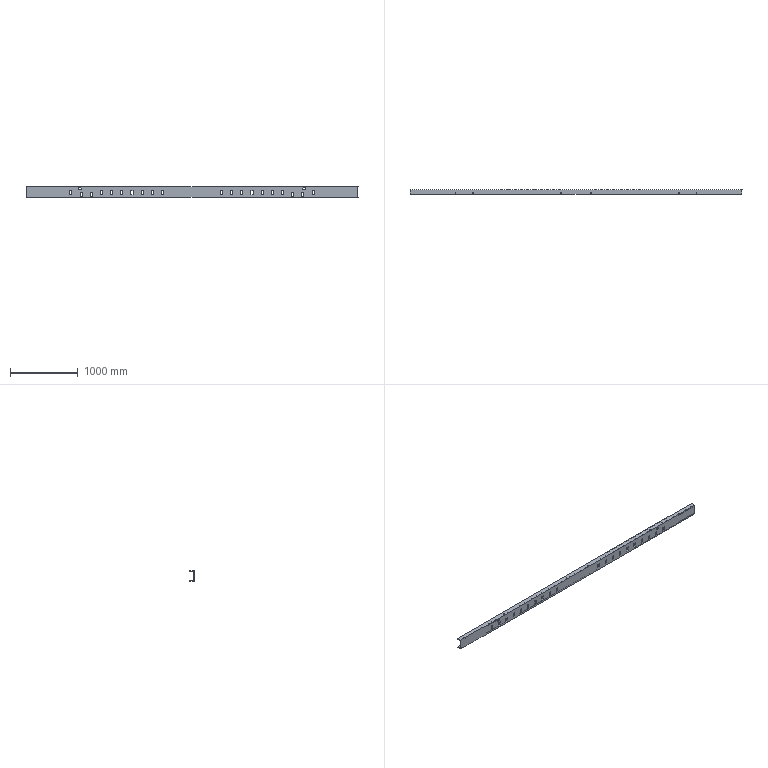Part | STEP file | 01-Channel 160x65(symmetric)_default<machining> | 1 solid | 114 faces | box 4896 x 65 x 160 mm | volume 11823421 mm3 | plane 92 | cylinder 22 | commonest cylinder face diameters 8.5 x12 20 x4 40 x4 10 x2